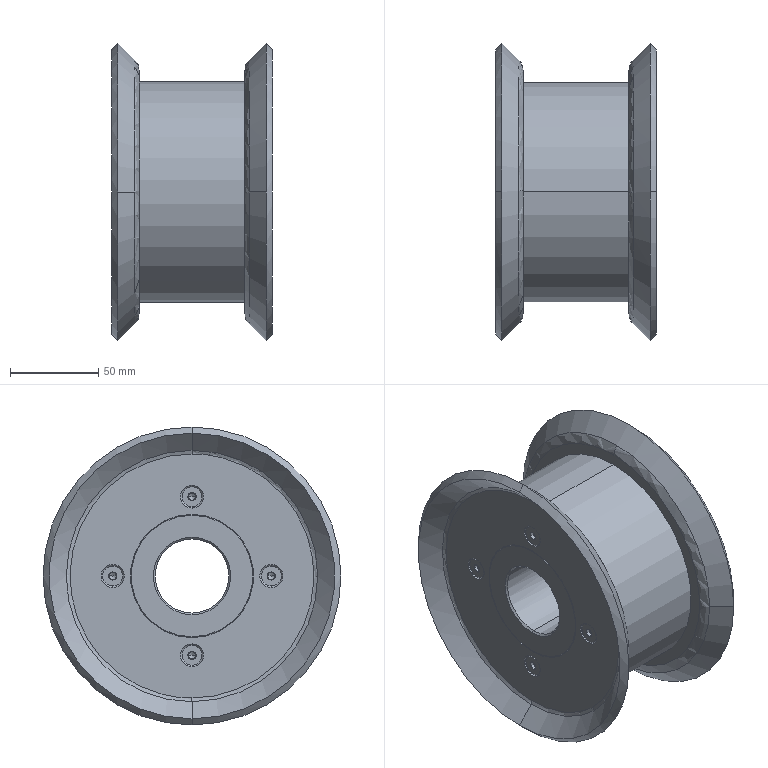Part | SolidWorks | 11 solids | 726 faces | box 91.113 x 169.042 x 169.042 mm | volume 833344 mm3 | cylinder 292 | cone 182 | plane 132 | spline 120 | commonest cylinder face diameters 6 x200 5 x16 6.6 x16 11.34 x16 13 x16 70 x8